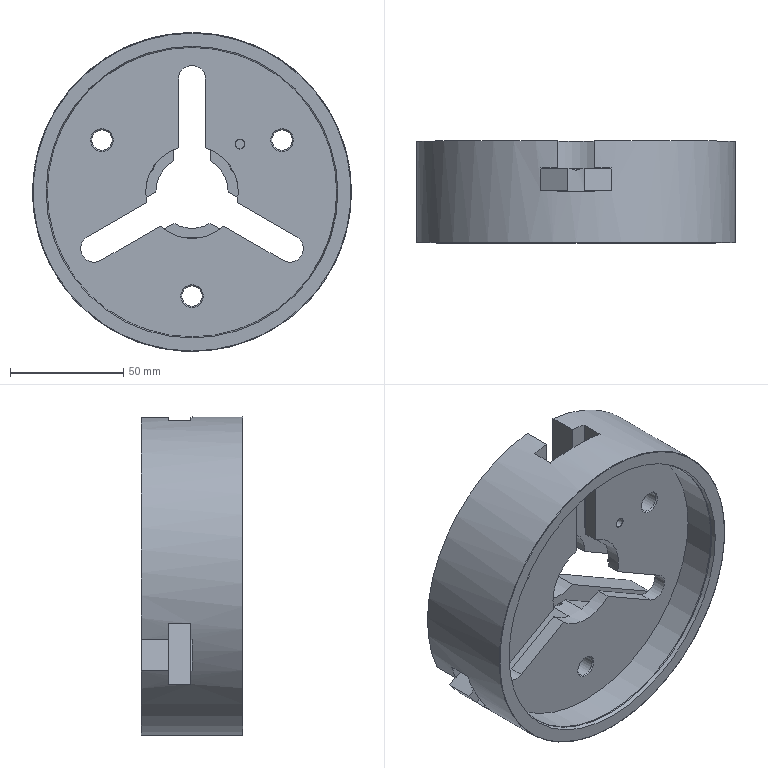NC program | NX | posted with a generic post | part box 141 x 45 x 141 mm
Whole program:
N10 G17 G21 G94 G90
(PLANAR_MILL_2_COPY_COPY_2 , TOOL : D30)
N12 T07 M6
N14 G54
N16 G17 G0 G90 X0. Y110. S0 M3
N18 G43 Z100. H7
N20 Z-20.
N22 G94 G1 Z-21. F250.
N24 Y80.
N26 X0.5
N28 Y15.
N30 X-0.5
N32 Y80.
N34 X0.
N36 Y110.
N38 Z-20.
N40 G0 Z-21.
N42 G1 Z-22.
N44 Y80.
N46 X0.5
N48 Y15.
N50 X-0.5
N52 Y80.
N54 X0.
N56 Y110.
N58 Z-21.
N60 G0 Z100.
(PLANAR_MILL_2_COPY_COPY_2_COPY , TOOL : D30)
N62 X-95.263 Y-55.
N64 Z-20.
N66 G1 Z-21.
N68 X-69.282 Y-40.
N70 X-69.532 Y-39.567
N72 X-13.24 Y-7.067
N74 X-12.74 Y-7.933
N76 X-69.032 Y-40.433
N78 X-69.282 Y-40.
N80 X-95.263 Y-55.
N82 Z-20.
N84 G0 Z-21.
N86 G1 Z-22.
N88 X-69.282 Y-40.
N90 X-69.532 Y-39.567
N92 X-13.24 Y-7.067
N94 X-12.74 Y-7.933
N96 X-69.032 Y-40.433
N98 X-69.282 Y-40.
N100 X-95.263 Y-55.
N102 Z-21.
N104 G0 Z100.
(PLANAR_MILL_2_COPY_COPY_2_COPY_1 , TOOL : D30)
N106 X95.263
N108 Z-20.
N110 G1 Z-21.
N112 X69.282 Y-40.
N114 X69.032 Y-40.433
N116 X12.74 Y-7.933
N118 X13.24 Y-7.067
N120 X69.532 Y-39.567
N122 X69.282 Y-40.
N124 X95.263 Y-55.
N126 Z-20.
N128 G0 Z-21.
N130 G1 Z-22.
N132 X69.282 Y-40.
N134 X69.032 Y-40.433
N136 X12.74 Y-7.933
N138 X13.24 Y-7.067
N140 X69.532 Y-39.567
N142 X69.282 Y-40.
N144 X95.263 Y-55.
N146 Z-21.
N148 G0 Z100.
N150 M5
N152 M2